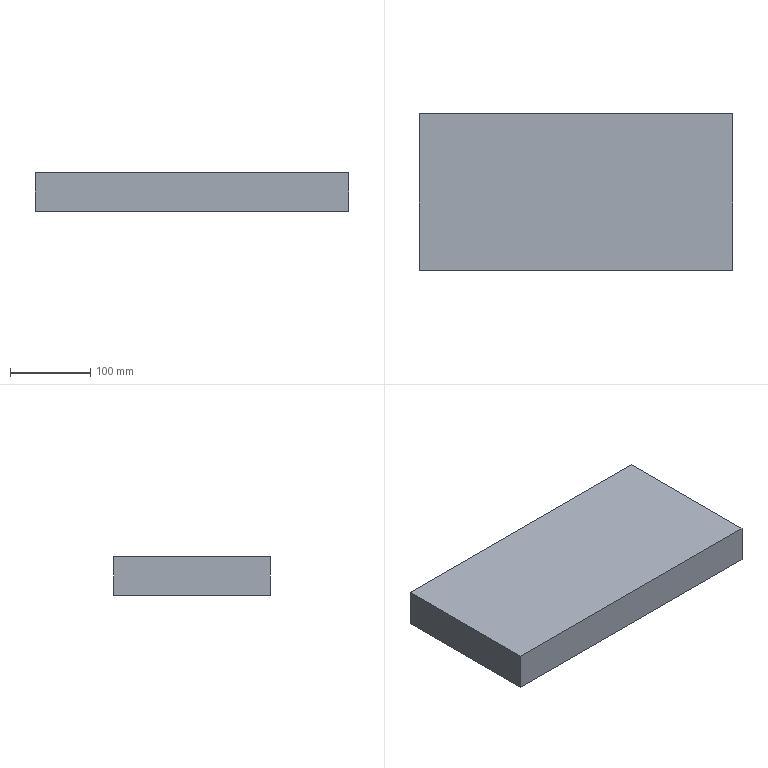Part | SolidWorks | features Extrusion 1, Shell 1 | 1 solid | 11 faces | box 390 x 195 x 47.5 mm | volume 741654 mm3 | plane 11
STEP:
#1=CARTESIAN_POINT('',(195.,0.,-23.75));
#2=VERTEX_POINT('',#1);
#3=CARTESIAN_POINT('',(-195.,0.,-23.75));
#4=VERTEX_POINT('',#3);
#5=CARTESIAN_POINT('',(-195.,0.,-23.75));
#6=DIRECTION('',(-1.,0.,0.));
#7=VECTOR('',#6,1000.);
#8=LINE('',#5,#7);
#9=EDGE_CURVE('',#2,#4,#8,.T.);
#10=ORIENTED_EDGE('',*,*,#9,.T.);
#11=CARTESIAN_POINT('',(-195.,195.,-23.75));
#12=VERTEX_POINT('',#11);
#13=CARTESIAN_POINT('',(-195.,195.,-23.75));
#14=DIRECTION('',(0.,-1.,0.));
#15=VECTOR('',#14,1000.);
#16=LINE('',#13,#15);
#17=EDGE_CURVE('',#12,#4,#16,.T.);
#18=ORIENTED_EDGE('',*,*,#17,.F.);
#19=CARTESIAN_POINT('',(195.,195.,-23.75));
#20=VERTEX_POINT('',#19);
#21=CARTESIAN_POINT('',(-195.,195.,-23.75));
#22=DIRECTION('',(-1.,0.,0.));
#23=VECTOR('',#22,1000.);
#24=LINE('',#21,#23);
#25=EDGE_CURVE('',#20,#12,#24,.T.);
#26=ORIENTED_EDGE('',*,*,#25,.F.);
#27=CARTESIAN_POINT('',(195.,195.,-23.75));
#28=DIRECTION('',(0.,-1.,0.));
#29=VECTOR('',#28,1000.);
#30=LINE('',#27,#29);
#31=EDGE_CURVE('',#20,#2,#30,.T.);
#32=ORIENTED_EDGE('',*,*,#31,.T.);
#33=EDGE_LOOP('',(#10,#18,#26,#32));
#34=FACE_OUTER_BOUND('',#33,.T.);
#35=CARTESIAN_POINT('',(189.,6.,-23.75));
#36=VERTEX_POINT('',#35);
#37=CARTESIAN_POINT('',(-189.,6.,-23.75));
#38=VERTEX_POINT('',#37);
#39=CARTESIAN_POINT('',(-195.,6.,-23.75));
#40=DIRECTION('',(-1.,0.,0.));
#41=VECTOR('',#40,1000.);
#42=LINE('',#39,#41);
#43=EDGE_CURVE('',#36,#38,#42,.T.);
#44=ORIENTED_EDGE('',*,*,#43,.F.);
#45=CARTESIAN_POINT('',(189.,189.,-23.75));
#46=VERTEX_POINT('',#45);
#47=CARTESIAN_POINT('',(189.,195.,-23.75));
#48=DIRECTION('',(0.,-1.,0.));
#49=VECTOR('',#48,1000.);
#50=LINE('',#47,#49);
#51=EDGE_CURVE('',#46,#36,#50,.T.);
#52=ORIENTED_EDGE('',*,*,#51,.F.);
#53=CARTESIAN_POINT('',(-189.,189.,-23.75));
#54=VERTEX_POINT('',#53);
#55=CARTESIAN_POINT('',(-195.,189.,-23.75));
#56=DIRECTION('',(-1.,0.,0.));
#57=VECTOR('',#56,1000.);
#58=LINE('',#55,#57);
#59=EDGE_CURVE('',#46,#54,#58,.T.);
#60=ORIENTED_EDGE('',*,*,#59,.T.);
#61=CARTESIAN_POINT('',(-189.,195.,-23.75));
#62=DIRECTION('',(0.,-1.,0.));
#63=VECTOR('',#62,1000.);
#64=LINE('',#61,#63);
#65=EDGE_CURVE('',#54,#38,#64,.T.);
#66=ORIENTED_EDGE('',*,*,#65,.T.);
#67=EDGE_LOOP('',(#44,#52,#60,#66));
#68=FACE_BOUND('',#67,.T.);
#69=CARTESIAN_POINT('',(-195.,195.,-23.75));
#70=DIRECTION('',(0.,0.,1.));
#71=DIRECTION('',(1.,0.,0.));
#72=AXIS2_PLACEMENT_3D('',#69,#70,#71);
#73=PLANE('',#72);
#74=ADVANCED_FACE('',(#34,#68),#73,.F.);
#75=CARTESIAN_POINT('',(195.,0.,23.75));
#76=VERTEX_POINT('',#75);
#77=CARTESIAN_POINT('',(195.,0.,-23.75));
#78=DIRECTION('',(0.,0.,-1.));
#79=VECTOR('',#78,1000.);
#80=LINE('',#77,#79);
#81=EDGE_CURVE('',#76,#2,#80,.T.);
#82=ORIENTED_EDGE('',*,*,#81,.T.);
#83=ORIENTED_EDGE('',*,*,#31,.F.);
#84=CARTESIAN_POINT('',(195.,195.,23.75));
#85=VERTEX_POINT('',#84);
#86=CARTESIAN_POINT('',(195.,195.,-23.75));
#87=DIRECTION('',(0.,0.,-1.));
#88=VECTOR('',#87,1000.);
#89=LINE('',#86,#88);
#90=EDGE_CURVE('',#85,#20,#89,.T.);
#91=ORIENTED_EDGE('',*,*,#90,.F.);
#92=CARTESIAN_POINT('',(195.,195.,23.75));
#93=DIRECTION('',(0.,-1.,0.));
#94=VECTOR('',#93,1000.);
#95=LINE('',#92,#94);
#96=EDGE_CURVE('',#85,#76,#95,.T.);
#97=ORIENTED_EDGE('',*,*,#96,.T.);
#98=EDGE_LOOP('',(#82,#83,#91,#97));
#99=FACE_OUTER_BOUND('',#98,.T.);
#100=CARTESIAN_POINT('',(195.,195.,-23.75));
#101=DIRECTION('',(-1.,0.,0.));
#102=DIRECTION('',(0.,0.,1.));
#103=AXIS2_PLACEMENT_3D('',#100,#101,#102);
#104=PLANE('',#103);
#105=ADVANCED_FACE('',(#99),#104,.F.);
#106=CARTESIAN_POINT('',(-195.,0.,23.75));
#107=VERTEX_POINT('',#106);
#108=CARTESIAN_POINT('',(-195.,0.,-23.75));
#109=DIRECTION('',(0.,0.,1.));
#110=VECTOR('',#109,1000.);
#111=LINE('',#108,#110);
#112=EDGE_CURVE('',#4,#107,#111,.T.);
#113=ORIENTED_EDGE('',*,*,#112,.T.);
#114=CARTESIAN_POINT('',(-195.,195.,23.75));
#115=VERTEX_POINT('',#114);
#116=CARTESIAN_POINT('',(-195.,195.,23.75));
#117=DIRECTION('',(0.,-1.,0.));
#118=VECTOR('',#117,1000.);
#119=LINE('',#116,#118);
#120=EDGE_CURVE('',#115,#107,#119,.T.);
#121=ORIENTED_EDGE('',*,*,#120,.F.);
#122=CARTESIAN_POINT('',(-195.,195.,-23.75));
#123=DIRECTION('',(0.,0.,1.));
#124=VECTOR('',#123,1000.);
#125=LINE('',#122,#124);
#126=EDGE_CURVE('',#12,#115,#125,.T.);
#127=ORIENTED_EDGE('',*,*,#126,.F.);
#128=ORIENTED_EDGE('',*,*,#17,.T.);
#129=EDGE_LOOP('',(#113,#121,#127,#128));
#130=FACE_OUTER_BOUND('',#129,.T.);
#131=CARTESIAN_POINT('',(-195.,195.,-23.75));
#132=DIRECTION('',(1.,0.,0.));
#133=DIRECTION('',(0.,0.,-1.));
#134=AXIS2_PLACEMENT_3D('',#131,#132,#133);
#135=PLANE('',#134);
#136=ADVANCED_FACE('',(#130),#135,.F.);
#137=CARTESIAN_POINT('',(-195.,0.,23.75));
#138=DIRECTION('',(1.,0.,0.));
#139=VECTOR('',#138,1000.);
#140=LINE('',#137,#139);
#141=EDGE_CURVE('',#107,#76,#140,.T.);
#142=ORIENTED_EDGE('',*,*,#141,.T.);
#143=ORIENTED_EDGE('',*,*,#96,.F.);
#144=CARTESIAN_POINT('',(-195.,195.,23.75));
#145=DIRECTION('',(1.,0.,0.));
#146=VECTOR('',#145,1000.);
#147=LINE('',#144,#146);
#148=EDGE_CURVE('',#115,#85,#147,.T.);
#149=ORIENTED_EDGE('',*,*,#148,.F.);
#150=ORIENTED_EDGE('',*,*,#120,.T.);
#151=EDGE_LOOP('',(#142,#143,#149,#150));
#152=FACE_OUTER_BOUND('',#151,.T.);
#153=CARTESIAN_POINT('',(-195.,195.,23.75));
#154=DIRECTION('',(0.,0.,-1.));
#155=DIRECTION('',(-1.,0.,0.));
#156=AXIS2_PLACEMENT_3D('',#153,#154,#155);
#157=PLANE('',#156);
#158=ADVANCED_FACE('',(#152),#157,.F.);
#159=ORIENTED_EDGE('',*,*,#90,.T.);
#160=ORIENTED_EDGE('',*,*,#25,.T.);
#161=ORIENTED_EDGE('',*,*,#126,.T.);
#162=ORIENTED_EDGE('',*,*,#148,.T.);
#163=EDGE_LOOP('',(#159,#160,#161,#162));
#164=FACE_OUTER_BOUND('',#163,.T.);
#165=CARTESIAN_POINT('',(0.,195.,0.));
#166=DIRECTION('',(0.,1.,0.));
#167=DIRECTION('',(0.,0.,1.));
#168=AXIS2_PLACEMENT_3D('',#165,#166,#167);
#169=PLANE('',#168);
#170=ADVANCED_FACE('',(#164),#169,.T.);
#171=ORIENTED_EDGE('',*,*,#81,.F.);
#172=ORIENTED_EDGE('',*,*,#141,.F.);
#173=ORIENTED_EDGE('',*,*,#112,.F.);
#174=ORIENTED_EDGE('',*,*,#9,.F.);
#175=EDGE_LOOP('',(#171,#172,#173,#174));
#176=FACE_OUTER_BOUND('',#175,.T.);
#177=CARTESIAN_POINT('',(0.,0.,0.));
#178=DIRECTION('',(0.,1.,0.));
#179=DIRECTION('',(0.,0.,1.));
#180=AXIS2_PLACEMENT_3D('',#177,#178,#179);
#181=PLANE('',#180);
#182=ADVANCED_FACE('',(#176),#181,.F.);
#183=CARTESIAN_POINT('',(189.,6.,17.75));
#184=VERTEX_POINT('',#183);
#185=CARTESIAN_POINT('',(189.,6.,-23.75));
#186=DIRECTION('',(0.,0.,-1.));
#187=VECTOR('',#186,1000.);
#188=LINE('',#185,#187);
#189=EDGE_CURVE('',#184,#36,#188,.T.);
#190=ORIENTED_EDGE('',*,*,#189,.F.);
#191=CARTESIAN_POINT('',(189.,189.,17.75));
#192=VERTEX_POINT('',#191);
#193=CARTESIAN_POINT('',(189.,195.,17.75));
#194=DIRECTION('',(0.,-1.,0.));
#195=VECTOR('',#194,1000.);
#196=LINE('',#193,#195);
#197=EDGE_CURVE('',#192,#184,#196,.T.);
#198=ORIENTED_EDGE('',*,*,#197,.F.);
#199=CARTESIAN_POINT('',(189.,189.,-23.75));
#200=DIRECTION('',(0.,0.,-1.));
#201=VECTOR('',#200,1000.);
#202=LINE('',#199,#201);
#203=EDGE_CURVE('',#192,#46,#202,.T.);
#204=ORIENTED_EDGE('',*,*,#203,.T.);
#205=ORIENTED_EDGE('',*,*,#51,.T.);
#206=EDGE_LOOP('',(#190,#198,#204,#205));
#207=FACE_OUTER_BOUND('',#206,.T.);
#208=CARTESIAN_POINT('',(189.,195.,-23.75));
#209=DIRECTION('',(-1.,0.,0.));
#210=DIRECTION('',(0.,0.,1.));
#211=AXIS2_PLACEMENT_3D('',#208,#209,#210);
#212=PLANE('',#211);
#213=ADVANCED_FACE('',(#207),#212,.T.);
#214=CARTESIAN_POINT('',(-189.,6.,17.75));
#215=VERTEX_POINT('',#214);
#216=CARTESIAN_POINT('',(-189.,6.,-23.75));
#217=DIRECTION('',(0.,0.,1.));
#218=VECTOR('',#217,1000.);
#219=LINE('',#216,#218);
#220=EDGE_CURVE('',#38,#215,#219,.T.);
#221=ORIENTED_EDGE('',*,*,#220,.F.);
#222=ORIENTED_EDGE('',*,*,#65,.F.);
#223=CARTESIAN_POINT('',(-189.,189.,17.75));
#224=VERTEX_POINT('',#223);
#225=CARTESIAN_POINT('',(-189.,189.,-23.75));
#226=DIRECTION('',(0.,0.,1.));
#227=VECTOR('',#226,1000.);
#228=LINE('',#225,#227);
#229=EDGE_CURVE('',#54,#224,#228,.T.);
#230=ORIENTED_EDGE('',*,*,#229,.T.);
#231=CARTESIAN_POINT('',(-189.,195.,17.75));
#232=DIRECTION('',(0.,-1.,0.));
#233=VECTOR('',#232,1000.);
#234=LINE('',#231,#233);
#235=EDGE_CURVE('',#224,#215,#234,.T.);
#236=ORIENTED_EDGE('',*,*,#235,.T.);
#237=EDGE_LOOP('',(#221,#222,#230,#236));
#238=FACE_OUTER_BOUND('',#237,.T.);
#239=CARTESIAN_POINT('',(-189.,195.,-23.75));
#240=DIRECTION('',(1.,0.,0.));
#241=DIRECTION('',(0.,0.,-1.));
#242=AXIS2_PLACEMENT_3D('',#239,#240,#241);
#243=PLANE('',#242);
#244=ADVANCED_FACE('',(#238),#243,.T.);
#245=CARTESIAN_POINT('',(-195.,6.,17.75));
#246=DIRECTION('',(1.,0.,0.));
#247=VECTOR('',#246,1000.);
#248=LINE('',#245,#247);
#249=EDGE_CURVE('',#215,#184,#248,.T.);
#250=ORIENTED_EDGE('',*,*,#249,.F.);
#251=ORIENTED_EDGE('',*,*,#235,.F.);
#252=CARTESIAN_POINT('',(-195.,189.,17.75));
#253=DIRECTION('',(1.,0.,0.));
#254=VECTOR('',#253,1000.);
#255=LINE('',#252,#254);
#256=EDGE_CURVE('',#224,#192,#255,.T.);
#257=ORIENTED_EDGE('',*,*,#256,.T.);
#258=ORIENTED_EDGE('',*,*,#197,.T.);
#259=EDGE_LOOP('',(#250,#251,#257,#258));
#260=FACE_OUTER_BOUND('',#259,.T.);
#261=CARTESIAN_POINT('',(-195.,195.,17.75));
#262=DIRECTION('',(0.,0.,-1.));
#263=DIRECTION('',(-1.,0.,0.));
#264=AXIS2_PLACEMENT_3D('',#261,#262,#263);
#265=PLANE('',#264);
#266=ADVANCED_FACE('',(#260),#265,.T.);
#267=ORIENTED_EDGE('',*,*,#203,.F.);
#268=ORIENTED_EDGE('',*,*,#256,.F.);
#269=ORIENTED_EDGE('',*,*,#229,.F.);
#270=ORIENTED_EDGE('',*,*,#59,.F.);
#271=EDGE_LOOP('',(#267,#268,#269,#270));
#272=FACE_OUTER_BOUND('',#271,.T.);
#273=CARTESIAN_POINT('',(0.,189.,0.));
#274=DIRECTION('',(0.,1.,0.));
#275=DIRECTION('',(0.,0.,1.));
#276=AXIS2_PLACEMENT_3D('',#273,#274,#275);
#277=PLANE('',#276);
#278=ADVANCED_FACE('',(#272),#277,.F.);
#279=ORIENTED_EDGE('',*,*,#189,.T.);
#280=ORIENTED_EDGE('',*,*,#43,.T.);
#281=ORIENTED_EDGE('',*,*,#220,.T.);
#282=ORIENTED_EDGE('',*,*,#249,.T.);
#283=EDGE_LOOP('',(#279,#280,#281,#282));
#284=FACE_OUTER_BOUND('',#283,.T.);
#285=CARTESIAN_POINT('',(0.,6.,0.));
#286=DIRECTION('',(0.,1.,0.));
#287=DIRECTION('',(0.,0.,1.));
#288=AXIS2_PLACEMENT_3D('',#285,#286,#287);
#289=PLANE('',#288);
#290=ADVANCED_FACE('',(#284),#289,.T.);
#291=CLOSED_SHELL('',(#74,#105,#136,#158,#170,#182,#213,#244,#266,#278,#290));
#292=MANIFOLD_SOLID_BREP('',#291);
#293=CARTESIAN_POINT('',(0.,0.,0.));
#294=DIRECTION('',(0.,0.,1.));
#295=DIRECTION('',(1.,0.,0.));
#296=AXIS2_PLACEMENT_3D('',#293,#294,#295);
#297=(LENGTH_UNIT()NAMED_UNIT(*)SI_UNIT(.MILLI.,.METRE.));
#298=UNCERTAINTY_MEASURE_WITH_UNIT(LENGTH_MEASURE(0.00001),#297,'','');
#299=(NAMED_UNIT(*)PLANE_ANGLE_UNIT()SI_UNIT($,.RADIAN.));
#300=(NAMED_UNIT(*)SI_UNIT($,.STERADIAN.)SOLID_ANGLE_UNIT());
#301=(GEOMETRIC_REPRESENTATION_CONTEXT(3)GLOBAL_UNCERTAINTY_ASSIGNED_CONTEXT((#298))GLOBAL_UNIT_ASSIGNED_CONTEXT((#297,#299,#300))REPRESENTATION_CONTEXT('',''));
#302=ADVANCED_BREP_SHAPE_REPRESENTATION('',(#292,#296),#301);